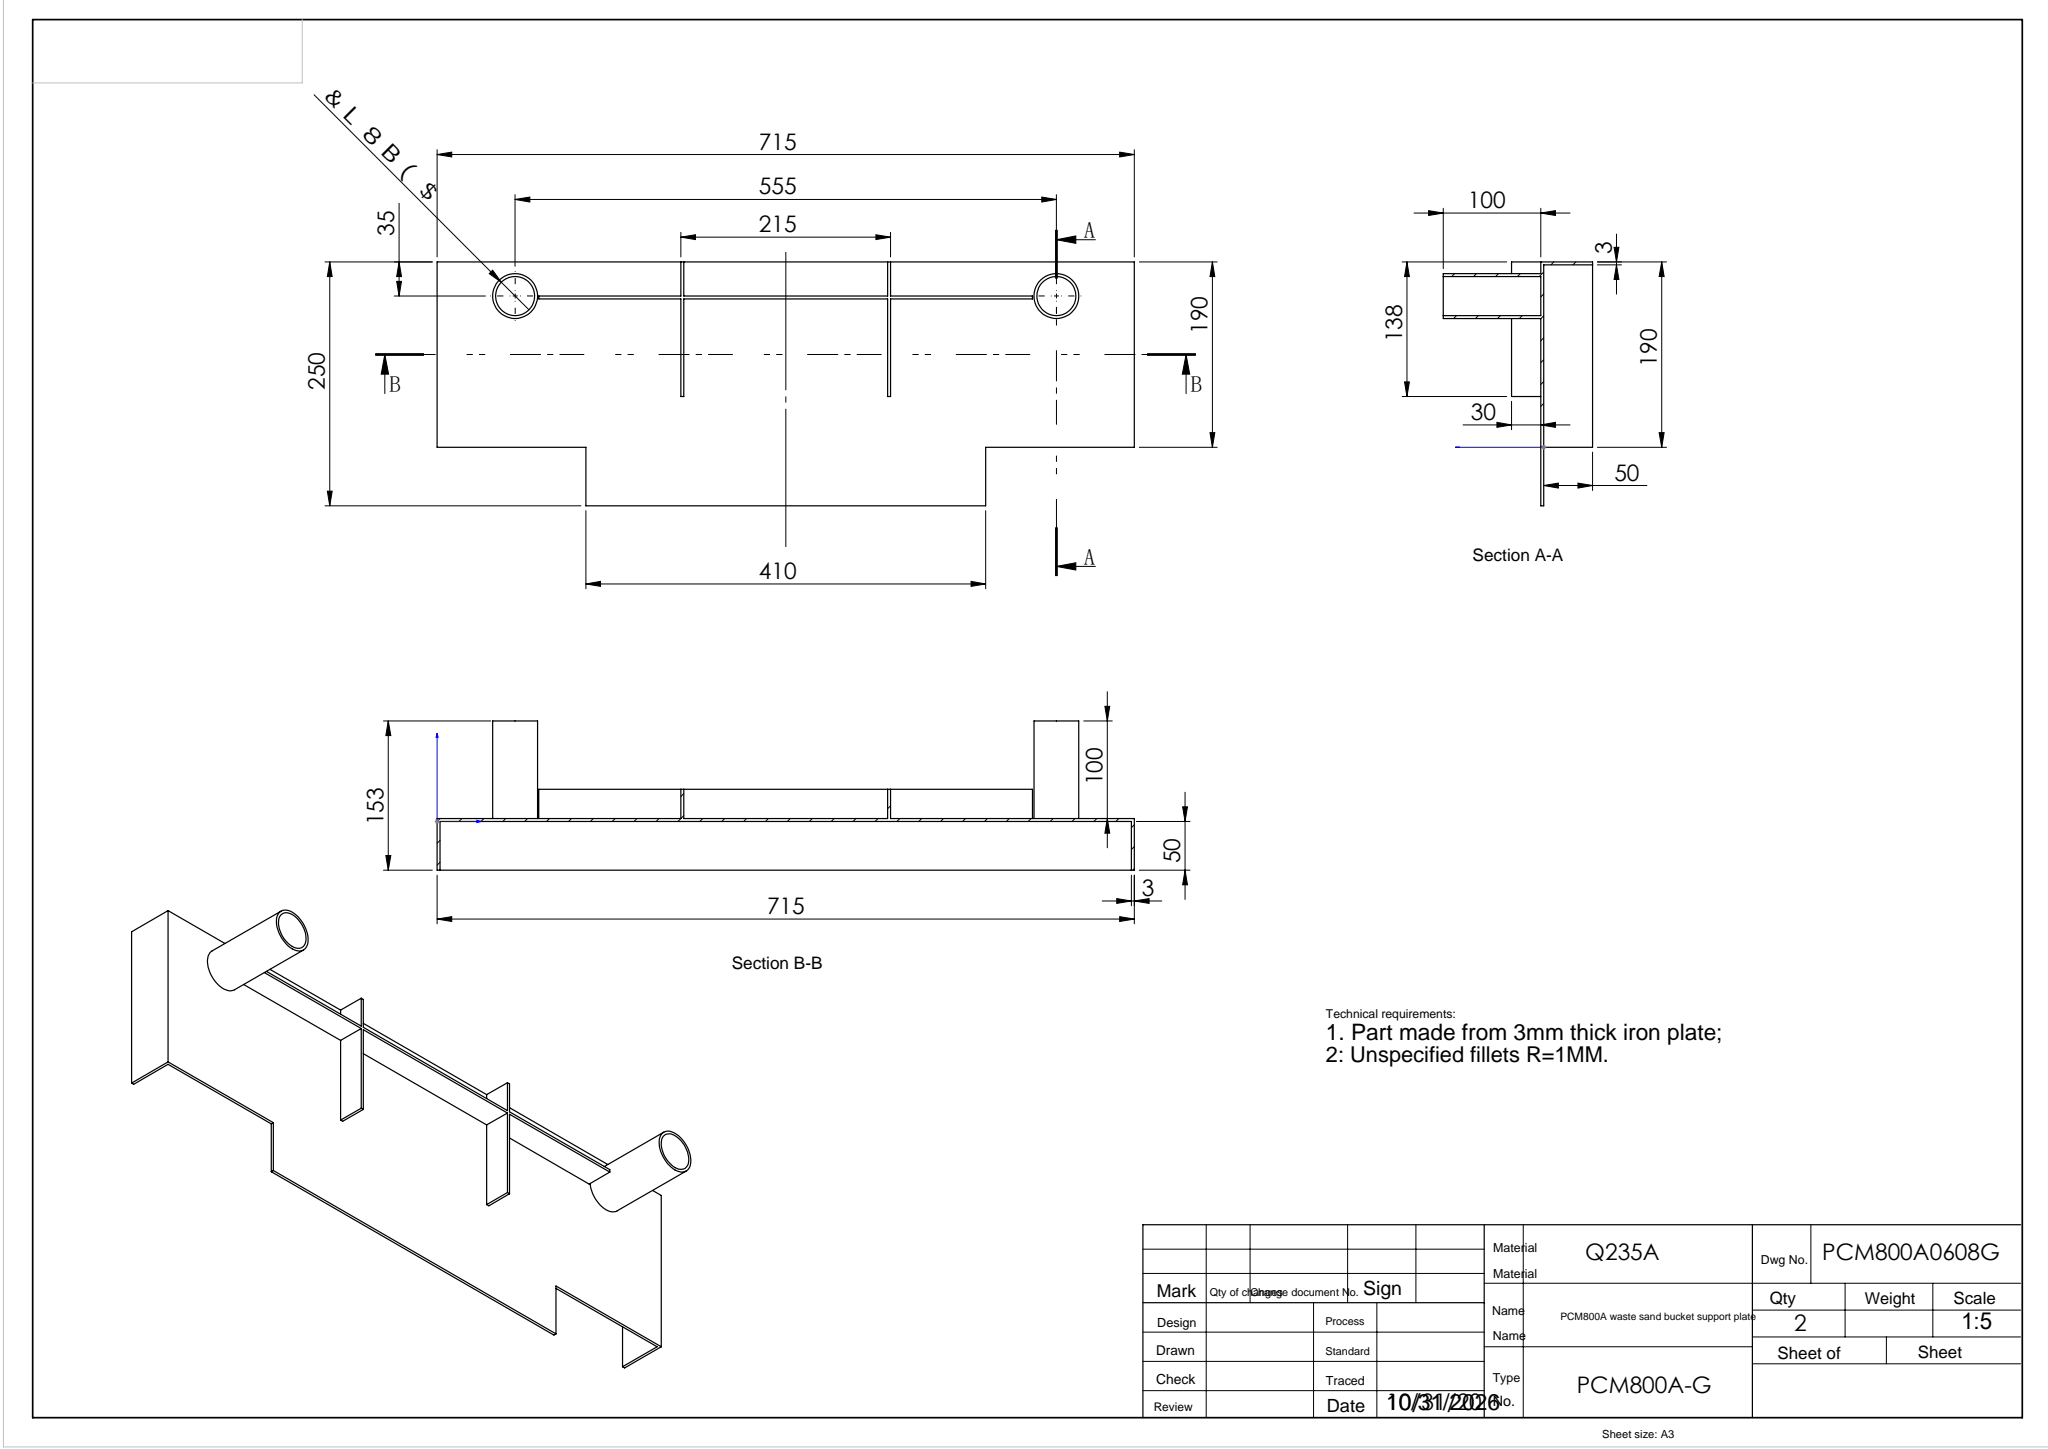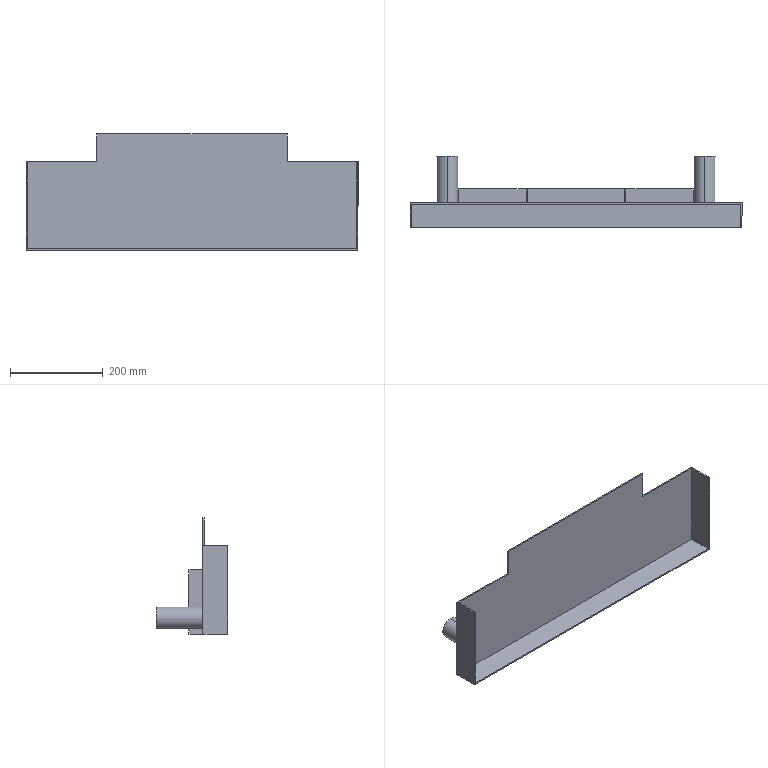Part | SolidWorks | features ICE 5, Extrusion 1 | 1 solid | 46 faces | box 715 x 153 x 250 mm | volume 795621 mm3 | plane 38 | cylinder 8 | commonest cylinder face diameters 40 x4 46 x4